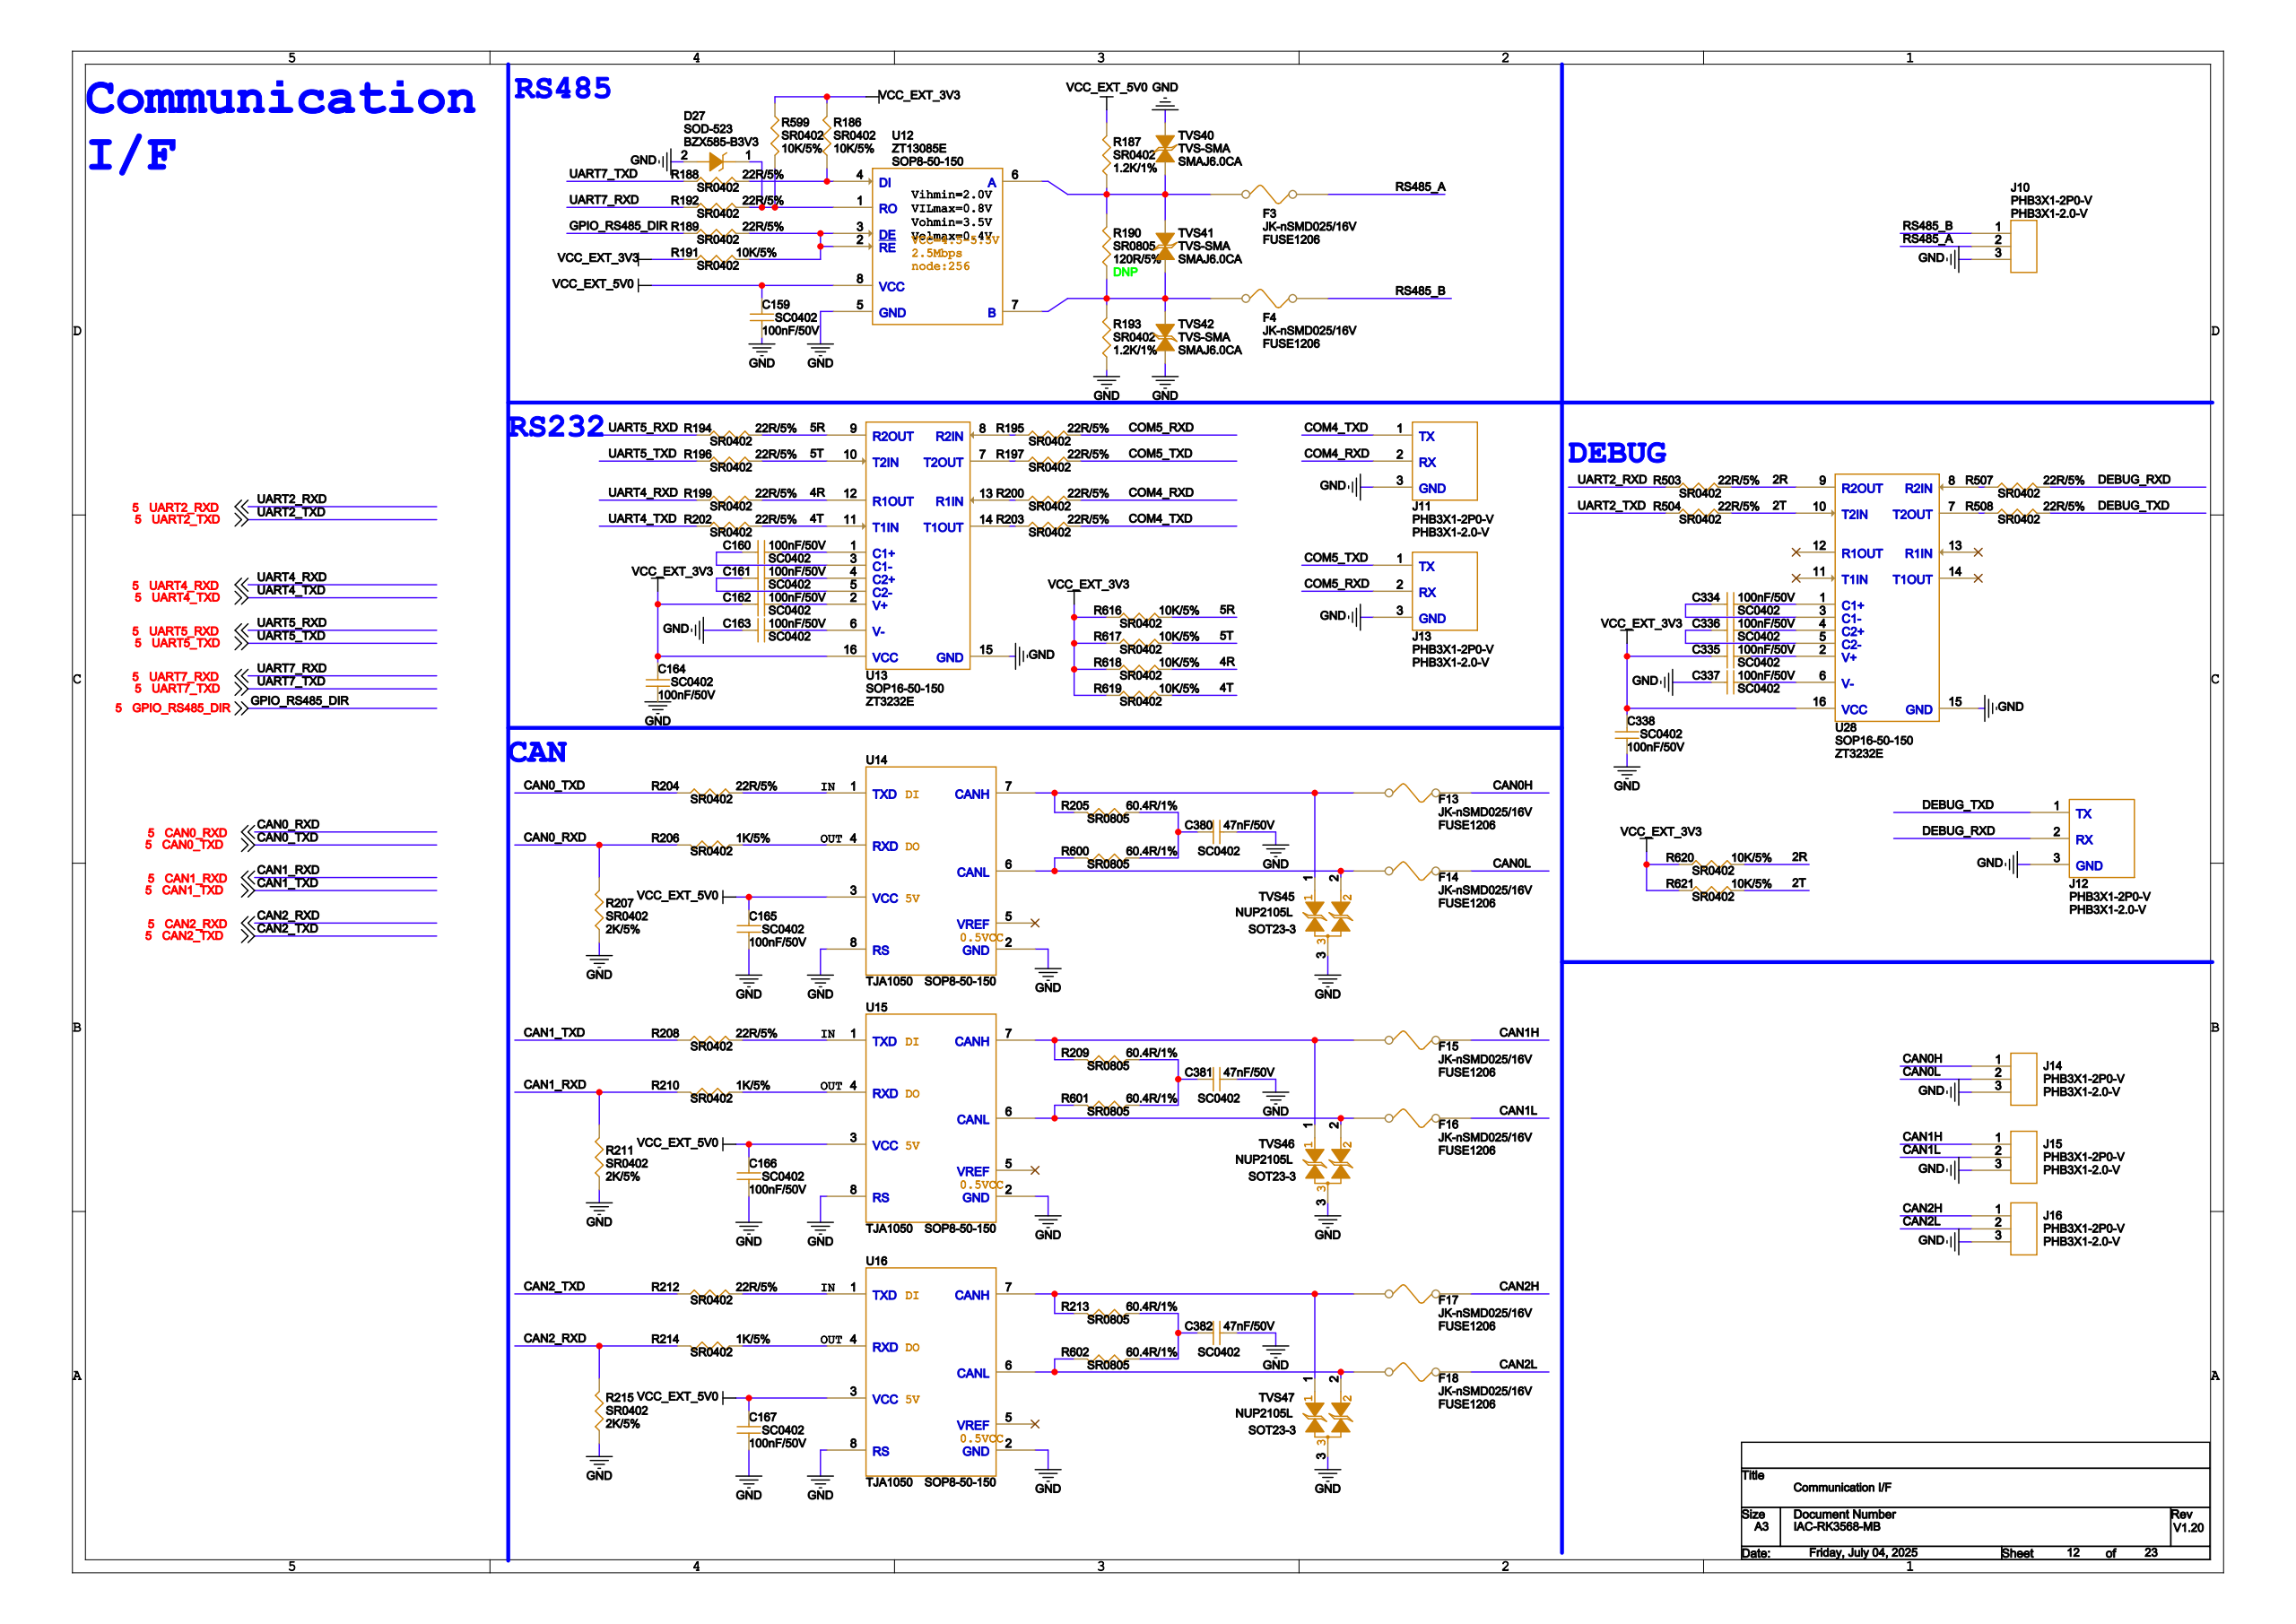Circuit board | Cadence Allegro | 1138 parts | 722 nets | one sheet of the schematic
Parts on this sheet (reference | value | footprint):
C159 | 100nF/50V | SC0402
C160 | 100nF/50V | SC0402
C161 | 100nF/50V | SC0402
C162 | 100nF/50V | SC0402
C163 | 100nF/50V | SC0402
C164 | 100nF/50V | SC0402
C165 | 100nF/50V | SC0402
C166 | 100nF/50V | SC0402
C167 | 100nF/50V | SC0402
C334 | 100nF/50V | SC0402
C335 | 100nF/50V | SC0402
C336 | 100nF/50V | SC0402
C337 | 100nF/50V | SC0402
C338 | 100nF/50V | SC0402
C380 | 47nF/50V | SC0402
C381 | 47nF/50V | SC0402
C382 | 47nF/50V | SC0402
D27 | BZX585-B3V3 | SOD-523
F3 | JK-nSMD025/16V | FUSE1206
F4 | JK-nSMD025/16V | FUSE1206
F13 | JK-nSMD025/16V | FUSE1206
F14 | JK-nSMD025/16V | FUSE1206
F15 | JK-nSMD025/16V | FUSE1206
F16 | JK-nSMD025/16V | FUSE1206
F17 | JK-nSMD025/16V | FUSE1206
F18 | JK-nSMD025/16V | FUSE1206
J10 | PHB3X1-2.0-V | PHB3X1-2P0-V
J11 | PHB3X1-2.0-V | PHB3X1-2P0-V
J12 | PHB3X1-2.0-V | PHB3X1-2P0-V
J13 | PHB3X1-2.0-V | PHB3X1-2P0-V
J14 | PHB3X1-2.0-V | PHB3X1-2P0-V
J15 | PHB3X1-2.0-V | PHB3X1-2P0-V
J16 | PHB3X1-2.0-V | PHB3X1-2P0-V
R186 | 10K/5% | SR0402
R187 | 1.2K/1% | SR0402
R188 | 22R/5% | SR0402
R189 | 22R/5% | SR0402
R190 | 120R/5% | SR0805
R191 | 10K/5% | SR0402
R192 | 22R/5% | SR0402
R193 | 1.2K/1% | SR0402
R194 | 22R/5% | SR0402
R195 | 22R/5% | SR0402
R196 | 22R/5% | SR0402
R197 | 22R/5% | SR0402
R199 | 22R/5% | SR0402
R200 | 22R/5% | SR0402
R202 | 22R/5% | SR0402
R203 | 22R/5% | SR0402
R204 | 22R/5% | SR0402
R205 | 60.4R/1% | SR0805
R206 | 1K/5% | SR0402
R207 | 2K/5% | SR0402
R208 | 22R/5% | SR0402
R209 | 60.4R/1% | SR0805
R210 | 1K/5% | SR0402
R211 | 2K/5% | SR0402
R212 | 22R/5% | SR0402
R213 | 60.4R/1% | SR0805
R214 | 1K/5% | SR0402
R215 | 2K/5% | SR0402
R503 | 22R/5% | SR0402
R504 | 22R/5% | SR0402
R507 | 22R/5% | SR0402
R508 | 22R/5% | SR0402
R599 | 10K/5% | SR0402
R600 | 60.4R/1% | SR0805
R601 | 60.4R/1% | SR0805
R602 | 60.4R/1% | SR0805
R616 | 10K/5% | SR0402
R617 | 10K/5% | SR0402
R618 | 10K/5% | SR0402
R619 | 10K/5% | SR0402
R620 | 10K/5% | SR0402
R621 | 10K/5% | SR0402
TVS40 | SMAJ6.0CA | TVS-SMA
TVS41 | SMAJ6.0CA | TVS-SMA
TVS42 | SMAJ6.0CA | TVS-SMA
TVS45 | NUP2105L | SOT23-3
TVS46 | NUP2105L | SOT23-3
TVS47 | NUP2105L | SOT23-3
U12 | ZT13085E | SOP8-50-150
U13 | ZT3232E | SOP16-50-150
U14 | TJA1050 | SOP8-50-150
U15 | TJA1050 | SOP8-50-150
U16 | TJA1050 | SOP8-50-150
U28 | ZT3232E | SOP16-50-150
Nets of these parts (net: part-pin ...):
VCC_EXT_5V0: C159-1 C165-1 C166-1 C167-1 R187-2 U12-8 U14-3 U15-3 U16-3
VCC_EXT_3V3: C162-1 C164-2 C335-1 C338-2 R186-2 R191-1 R599-1 R616-1 R617-1 R618-1 R619-1 R620-1 R621-1 U13-16 U28-16
GND: C159-2 C163-1 C164-1 C165-2 C166-2 C167-2 C337-1 C338-1 C380-2 C381-2 C382-2 D27-2 J10-3 J11-3 J12-3 J13-3 J14-3 J15-3 J16-3 R193-1 R207-1 R211-1 R215-1 TVS40-2 TVS42-2 TVS45-3 TVS46-3 TVS47-3 U12-5 U13-15 U14-2 U14-8 U15-2 U15-8 U16-2 U16-8 U28-15
N6814118: C380-1 R205-1 R600-1
N6814408: C381-1 R209-1 R601-1
N6814641: C382-1 R213-1 R602-1
N4063610: F13-2 R205-2 TVS45-1 U14-7
N4671346: F15-2 R209-2 TVS46-1 U15-7
N4672117: F17-2 R213-2 TVS47-1 U16-7
N4063682: F14-2 R600-2 TVS45-2 U14-6
N4671320: F16-2 R601-2 TVS46-2 U15-6
N4672091: F18-2 R602-2 TVS47-2 U16-6
N4059877: D27-1 R192-2 R599-2 U12-1
CAN0H: F13-1 J14-1
CAN0L: F14-1 J14-2
CAN1H: F15-1 J15-1
CAN1L: F16-1 J15-2
CAN2H: F17-1 J16-1
CAN2L: F18-1 J16-2
RS485_A: F3-1 J10-2
N4059715: F3-2 R187-1 R190-2 TVS40-1 TVS41-2 U12-6
RS485_B: F4-1 J10-1
N4059703: F4-2 R190-1 R193-2 TVS41-1 TVS42-1 U12-7
CAN0_RXD: R206-2 R207-2
CAN1_RXD: R210-2 R211-2
CAN2_RXD: R214-2 R215-2
CAN0_TXD: R204-1
CAN1_TXD: R208-1
UART2_RXD: R503-1
UART2_TXD: R504-1
CAN2_TXD: R212-1
UART4_RXD: R199-1
UART4_TXD: R202-1
UART5_RXD: R194-1
GPIO_RS485_DIR: R189-1
UART5_TXD: R196-1
UART7_TXD: R188-1
UART7_RXD: R192-1
N4059873: R186-1 R188-2 U12-4
N4059579: R189-2 R191-2 U12-2 U12-3
N4059133: C160-2 U13-1
N4059117: C160-1 U13-3
N4059125: C161-2 U13-4
N4059109: C161-1 U13-5
N4059451: R200-1 U13-13
4R: R199-2 R618-2 U13-12
N4059459: R195-1 U13-8
5R: R194-2 R616-2 U13-9
4T: R202-2 R619-2 U13-11
N4059455: R203-1 U13-14
5T: R196-2 R617-2 U13-10
N4059447: R197-1 U13-7
N4059145: C162-2 U13-2
N4059149: C163-2 U13-6
N5395511: C334-2 U28-1
N5395495: C334-1 U28-3
N5395503: C336-2 U28-4
N5395487: C336-1 U28-5
N5395831: R507-1 U28-8
2R: R503-2 R620-2 U28-9
2T: R504-2 R621-2 U28-10
N5395819: R508-1 U28-7
N5395523: C335-2 U28-2
N5395527: C337-2 U28-6
N4063858: R206-1 U14-4
N4063828: R204-2 U14-1
N4671632: R210-1 U15-4
N4671602: R208-2 U15-1
N4672403: R214-1 U16-4
N4672373: R212-2 U16-1
COM4_TXD: J11-1 R203-2
COM4_RXD: J11-2 R200-2
DEBUG_RXD: J12-2 R507-2
DEBUG_TXD: J12-1 R508-2
COM5_TXD: J13-1 R197-2
COM5_RXD: J13-2 R195-2